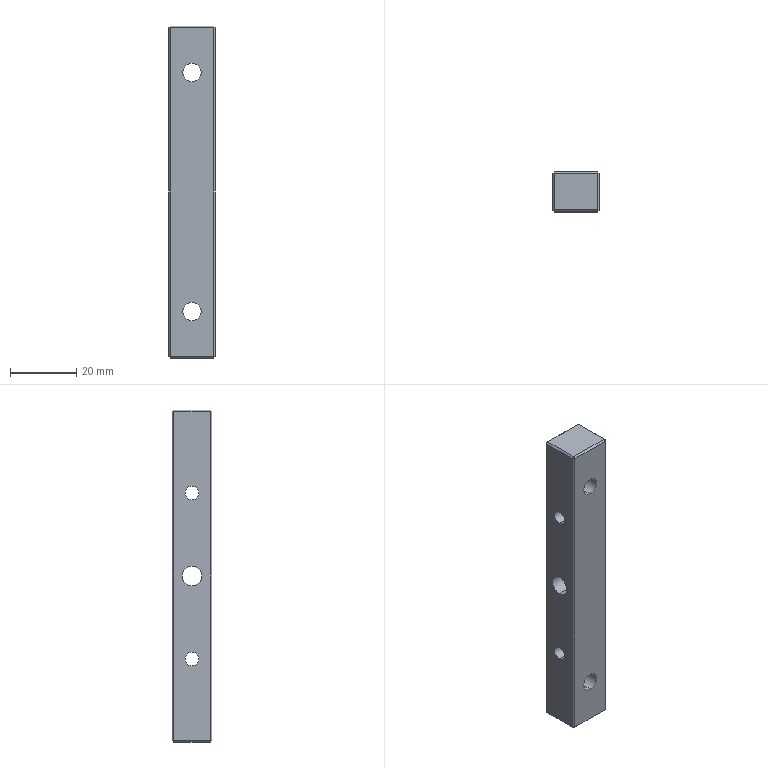Part | STEP file | ND25021-01-JDKM-19-TL | 1 solid | 42 faces | box 14 x 12 x 100 mm | volume 14792 mm3 | plane 28 | cylinder 14 | commonest cylinder face diameters 4.2 x4 5.5 x4 10 x4 6 x2